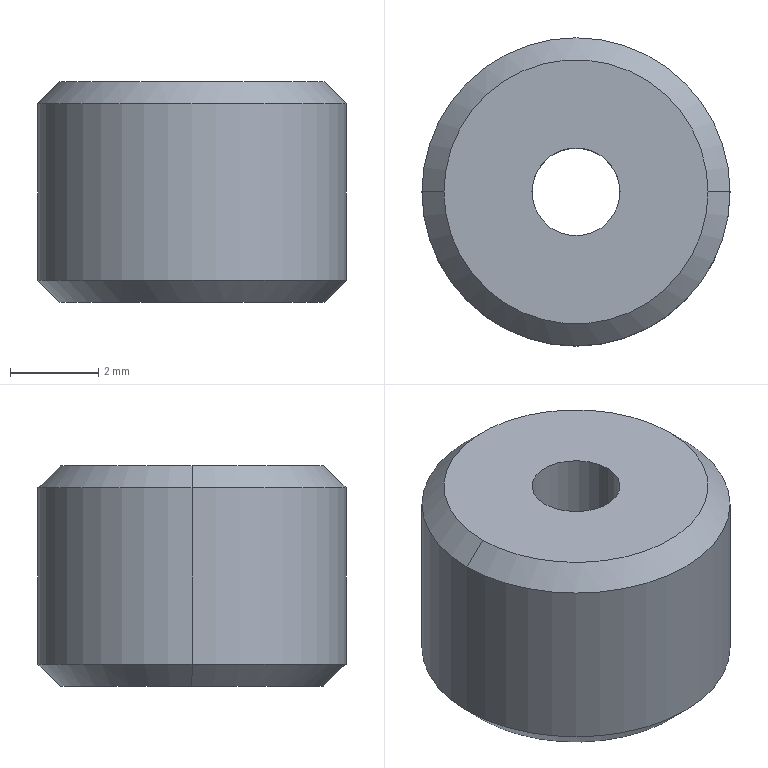Part | SolidWorks | features Chamfer 1, Extrusion 1, ICE 1 | 1 solid | 10 faces | box 7 x 7 x 5 mm | volume 171.479 mm3 | cone 4 | cylinder 4 | plane 2 | commonest cylinder face diameters 2 x2 7 x2
STEP:
#1=CARTESIAN_POINT('',(3.,0.,5.));
#2=VERTEX_POINT('',#1);
#3=CARTESIAN_POINT('',(-3.,0.,5.));
#4=VERTEX_POINT('',#3);
#5=CARTESIAN_POINT('',(0.,0.,5.));
#6=DIRECTION('',(0.,0.,1.));
#7=DIRECTION('',(1.,0.,0.));
#8=AXIS2_PLACEMENT_3D('',#5,#6,#7);
#9=CIRCLE('',#8,3.);
#10=EDGE_CURVE('',#2,#4,#9,.T.);
#11=ORIENTED_EDGE('',*,*,#10,.F.);
#12=CARTESIAN_POINT('',(3.5,0.,4.5));
#13=VERTEX_POINT('',#12);
#14=CARTESIAN_POINT('',(3.,0.,5.));
#15=DIRECTION('',(0.7071,0.,-0.7071));
#16=VECTOR('',#15,1000.);
#17=LINE('',#14,#16);
#18=EDGE_CURVE('',#2,#13,#17,.T.);
#19=ORIENTED_EDGE('',*,*,#18,.T.);
#20=CARTESIAN_POINT('',(-3.5,0.,4.5));
#21=VERTEX_POINT('',#20);
#22=CARTESIAN_POINT('',(0.,0.,4.5));
#23=DIRECTION('',(0.,0.,-1.));
#24=DIRECTION('',(1.,0.,0.));
#25=AXIS2_PLACEMENT_3D('',#22,#23,#24);
#26=CIRCLE('',#25,3.5);
#27=EDGE_CURVE('',#21,#13,#26,.T.);
#28=ORIENTED_EDGE('',*,*,#27,.F.);
#29=CARTESIAN_POINT('',(-3.,0.,5.));
#30=DIRECTION('',(-0.7071,0.,-0.7071));
#31=VECTOR('',#30,1000.);
#32=LINE('',#29,#31);
#33=EDGE_CURVE('',#4,#21,#32,.T.);
#34=ORIENTED_EDGE('',*,*,#33,.F.);
#35=EDGE_LOOP('',(#11,#19,#28,#34));
#36=FACE_OUTER_BOUND('',#35,.T.);
#37=CARTESIAN_POINT('',(0.,0.,5.));
#38=DIRECTION('',(0.,0.,-1.));
#39=DIRECTION('',(-1.,0.,0.));
#40=AXIS2_PLACEMENT_3D('',#37,#38,#39);
#41=CONICAL_SURFACE('',#40,3.,0.7854);
#42=ADVANCED_FACE('',(#36),#41,.T.);
#43=CARTESIAN_POINT('',(-3.,0.,0.));
#44=VERTEX_POINT('',#43);
#45=CARTESIAN_POINT('',(3.,0.,0.));
#46=VERTEX_POINT('',#45);
#47=CARTESIAN_POINT('',(0.,0.,0.));
#48=DIRECTION('',(0.,0.,-1.));
#49=DIRECTION('',(1.,0.,0.));
#50=AXIS2_PLACEMENT_3D('',#47,#48,#49);
#51=CIRCLE('',#50,3.);
#52=EDGE_CURVE('',#44,#46,#51,.T.);
#53=ORIENTED_EDGE('',*,*,#52,.F.);
#54=CARTESIAN_POINT('',(-3.5,0.,0.5));
#55=VERTEX_POINT('',#54);
#56=CARTESIAN_POINT('',(-3.5,0.,0.5));
#57=DIRECTION('',(-0.7071,0.,0.7071));
#58=VECTOR('',#57,1000.);
#59=LINE('',#56,#58);
#60=EDGE_CURVE('',#44,#55,#59,.T.);
#61=ORIENTED_EDGE('',*,*,#60,.T.);
#62=CARTESIAN_POINT('',(3.5,0.,0.5));
#63=VERTEX_POINT('',#62);
#64=CARTESIAN_POINT('',(0.,0.,0.5));
#65=DIRECTION('',(0.,0.,1.));
#66=DIRECTION('',(1.,0.,0.));
#67=AXIS2_PLACEMENT_3D('',#64,#65,#66);
#68=CIRCLE('',#67,3.5);
#69=EDGE_CURVE('',#63,#55,#68,.T.);
#70=ORIENTED_EDGE('',*,*,#69,.F.);
#71=CARTESIAN_POINT('',(3.5,0.,0.5));
#72=DIRECTION('',(0.7071,0.,0.7071));
#73=VECTOR('',#72,1000.);
#74=LINE('',#71,#73);
#75=EDGE_CURVE('',#46,#63,#74,.T.);
#76=ORIENTED_EDGE('',*,*,#75,.F.);
#77=EDGE_LOOP('',(#53,#61,#70,#76));
#78=FACE_OUTER_BOUND('',#77,.T.);
#79=CARTESIAN_POINT('',(0.,0.,0.5));
#80=DIRECTION('',(0.,0.,1.));
#81=DIRECTION('',(1.,0.,0.));
#82=AXIS2_PLACEMENT_3D('',#79,#80,#81);
#83=CONICAL_SURFACE('',#82,3.5,0.7854);
#84=ADVANCED_FACE('',(#78),#83,.T.);
#85=CARTESIAN_POINT('',(-1.,0.,0.));
#86=VERTEX_POINT('',#85);
#87=CARTESIAN_POINT('',(1.,0.,0.));
#88=VERTEX_POINT('',#87);
#89=CARTESIAN_POINT('',(0.,0.,0.));
#90=DIRECTION('',(0.,0.,1.));
#91=DIRECTION('',(1.,0.,0.));
#92=AXIS2_PLACEMENT_3D('',#89,#90,#91);
#93=CIRCLE('',#92,1.);
#94=EDGE_CURVE('',#86,#88,#93,.T.);
#95=ORIENTED_EDGE('',*,*,#94,.F.);
#96=CARTESIAN_POINT('',(-1.,0.,5.));
#97=VERTEX_POINT('',#96);
#98=CARTESIAN_POINT('',(-1.,0.,-6.));
#99=DIRECTION('',(0.,0.,1.));
#100=VECTOR('',#99,1000.);
#101=LINE('',#98,#100);
#102=EDGE_CURVE('',#86,#97,#101,.T.);
#103=ORIENTED_EDGE('',*,*,#102,.T.);
#104=CARTESIAN_POINT('',(1.,0.,5.));
#105=VERTEX_POINT('',#104);
#106=CARTESIAN_POINT('',(0.,0.,5.));
#107=DIRECTION('',(0.,0.,1.));
#108=DIRECTION('',(1.,0.,0.));
#109=AXIS2_PLACEMENT_3D('',#106,#107,#108);
#110=CIRCLE('',#109,1.);
#111=EDGE_CURVE('',#97,#105,#110,.T.);
#112=ORIENTED_EDGE('',*,*,#111,.T.);
#113=CARTESIAN_POINT('',(1.,0.,-6.));
#114=DIRECTION('',(0.,0.,1.));
#115=VECTOR('',#114,1000.);
#116=LINE('',#113,#115);
#117=EDGE_CURVE('',#88,#105,#116,.T.);
#118=ORIENTED_EDGE('',*,*,#117,.F.);
#119=EDGE_LOOP('',(#95,#103,#112,#118));
#120=FACE_OUTER_BOUND('',#119,.T.);
#121=CARTESIAN_POINT('',(0.,0.,-6.));
#122=DIRECTION('',(0.,0.,1.));
#123=DIRECTION('',(1.,0.,0.));
#124=AXIS2_PLACEMENT_3D('',#121,#122,#123);
#125=CYLINDRICAL_SURFACE('',#124,1.);
#126=ADVANCED_FACE('',(#120),#125,.F.);
#127=ORIENTED_EDGE('',*,*,#27,.T.);
#128=CARTESIAN_POINT('',(3.5,0.,5.));
#129=DIRECTION('',(0.,0.,-1.));
#130=VECTOR('',#129,1000.);
#131=LINE('',#128,#130);
#132=EDGE_CURVE('',#13,#63,#131,.T.);
#133=ORIENTED_EDGE('',*,*,#132,.T.);
#134=ORIENTED_EDGE('',*,*,#69,.T.);
#135=CARTESIAN_POINT('',(-3.5,0.,5.));
#136=DIRECTION('',(0.,0.,-1.));
#137=VECTOR('',#136,1000.);
#138=LINE('',#135,#137);
#139=EDGE_CURVE('',#21,#55,#138,.T.);
#140=ORIENTED_EDGE('',*,*,#139,.F.);
#141=EDGE_LOOP('',(#127,#133,#134,#140));
#142=FACE_OUTER_BOUND('',#141,.T.);
#143=CARTESIAN_POINT('',(0.,0.,5.));
#144=DIRECTION('',(0.,0.,-1.));
#145=DIRECTION('',(-1.,0.,0.));
#146=AXIS2_PLACEMENT_3D('',#143,#144,#145);
#147=CYLINDRICAL_SURFACE('',#146,3.5);
#148=ADVANCED_FACE('',(#142),#147,.T.);
#149=ORIENTED_EDGE('',*,*,#132,.F.);
#150=CARTESIAN_POINT('',(0.,0.,4.5));
#151=DIRECTION('',(0.,0.,-1.));
#152=DIRECTION('',(1.,0.,0.));
#153=AXIS2_PLACEMENT_3D('',#150,#151,#152);
#154=CIRCLE('',#153,3.5);
#155=EDGE_CURVE('',#13,#21,#154,.T.);
#156=ORIENTED_EDGE('',*,*,#155,.T.);
#157=ORIENTED_EDGE('',*,*,#139,.T.);
#158=CARTESIAN_POINT('',(0.,0.,0.5));
#159=DIRECTION('',(0.,0.,1.));
#160=DIRECTION('',(1.,0.,0.));
#161=AXIS2_PLACEMENT_3D('',#158,#159,#160);
#162=CIRCLE('',#161,3.5);
#163=EDGE_CURVE('',#55,#63,#162,.T.);
#164=ORIENTED_EDGE('',*,*,#163,.T.);
#165=EDGE_LOOP('',(#149,#156,#157,#164));
#166=FACE_OUTER_BOUND('',#165,.T.);
#167=CARTESIAN_POINT('',(0.,0.,5.));
#168=DIRECTION('',(0.,0.,-1.));
#169=DIRECTION('',(-1.,0.,0.));
#170=AXIS2_PLACEMENT_3D('',#167,#168,#169);
#171=CYLINDRICAL_SURFACE('',#170,3.5);
#172=ADVANCED_FACE('',(#166),#171,.T.);
#173=CARTESIAN_POINT('',(0.,0.,5.));
#174=DIRECTION('',(0.,0.,1.));
#175=DIRECTION('',(1.,0.,0.));
#176=AXIS2_PLACEMENT_3D('',#173,#174,#175);
#177=CIRCLE('',#176,3.);
#178=EDGE_CURVE('',#4,#2,#177,.T.);
#179=ORIENTED_EDGE('',*,*,#178,.T.);
#180=ORIENTED_EDGE('',*,*,#10,.T.);
#181=EDGE_LOOP('',(#179,#180));
#182=FACE_OUTER_BOUND('',#181,.T.);
#183=CARTESIAN_POINT('',(0.,0.,5.));
#184=DIRECTION('',(0.,0.,1.));
#185=DIRECTION('',(1.,0.,0.));
#186=AXIS2_PLACEMENT_3D('',#183,#184,#185);
#187=CIRCLE('',#186,1.);
#188=EDGE_CURVE('',#105,#97,#187,.T.);
#189=ORIENTED_EDGE('',*,*,#188,.F.);
#190=ORIENTED_EDGE('',*,*,#111,.F.);
#191=EDGE_LOOP('',(#189,#190));
#192=FACE_BOUND('',#191,.T.);
#193=CARTESIAN_POINT('',(0.,0.,5.));
#194=DIRECTION('',(0.,0.,1.));
#195=DIRECTION('',(1.,0.,0.));
#196=AXIS2_PLACEMENT_3D('',#193,#194,#195);
#197=PLANE('',#196);
#198=ADVANCED_FACE('',(#182,#192),#197,.T.);
#199=CARTESIAN_POINT('',(0.,0.,0.));
#200=DIRECTION('',(0.,0.,-1.));
#201=DIRECTION('',(1.,0.,0.));
#202=AXIS2_PLACEMENT_3D('',#199,#200,#201);
#203=CIRCLE('',#202,3.);
#204=EDGE_CURVE('',#46,#44,#203,.T.);
#205=ORIENTED_EDGE('',*,*,#204,.T.);
#206=ORIENTED_EDGE('',*,*,#52,.T.);
#207=EDGE_LOOP('',(#205,#206));
#208=FACE_OUTER_BOUND('',#207,.T.);
#209=CARTESIAN_POINT('',(0.,0.,0.));
#210=DIRECTION('',(0.,0.,1.));
#211=DIRECTION('',(1.,0.,0.));
#212=AXIS2_PLACEMENT_3D('',#209,#210,#211);
#213=CIRCLE('',#212,1.);
#214=EDGE_CURVE('',#88,#86,#213,.T.);
#215=ORIENTED_EDGE('',*,*,#214,.T.);
#216=ORIENTED_EDGE('',*,*,#94,.T.);
#217=EDGE_LOOP('',(#215,#216));
#218=FACE_BOUND('',#217,.T.);
#219=CARTESIAN_POINT('',(0.,0.,0.));
#220=DIRECTION('',(0.,0.,1.));
#221=DIRECTION('',(1.,0.,0.));
#222=AXIS2_PLACEMENT_3D('',#219,#220,#221);
#223=PLANE('',#222);
#224=ADVANCED_FACE('',(#208,#218),#223,.F.);
#225=ORIENTED_EDGE('',*,*,#102,.F.);
#226=ORIENTED_EDGE('',*,*,#214,.F.);
#227=ORIENTED_EDGE('',*,*,#117,.T.);
#228=ORIENTED_EDGE('',*,*,#188,.T.);
#229=EDGE_LOOP('',(#225,#226,#227,#228));
#230=FACE_OUTER_BOUND('',#229,.T.);
#231=CARTESIAN_POINT('',(0.,0.,-6.));
#232=DIRECTION('',(0.,0.,1.));
#233=DIRECTION('',(1.,0.,0.));
#234=AXIS2_PLACEMENT_3D('',#231,#232,#233);
#235=CYLINDRICAL_SURFACE('',#234,1.);
#236=ADVANCED_FACE('',(#230),#235,.F.);
#237=ORIENTED_EDGE('',*,*,#60,.F.);
#238=ORIENTED_EDGE('',*,*,#204,.F.);
#239=ORIENTED_EDGE('',*,*,#75,.T.);
#240=ORIENTED_EDGE('',*,*,#163,.F.);
#241=EDGE_LOOP('',(#237,#238,#239,#240));
#242=FACE_OUTER_BOUND('',#241,.T.);
#243=CARTESIAN_POINT('',(0.,0.,0.5));
#244=DIRECTION('',(0.,0.,1.));
#245=DIRECTION('',(1.,0.,0.));
#246=AXIS2_PLACEMENT_3D('',#243,#244,#245);
#247=CONICAL_SURFACE('',#246,3.5,0.7854);
#248=ADVANCED_FACE('',(#242),#247,.T.);
#249=ORIENTED_EDGE('',*,*,#18,.F.);
#250=ORIENTED_EDGE('',*,*,#178,.F.);
#251=ORIENTED_EDGE('',*,*,#33,.T.);
#252=ORIENTED_EDGE('',*,*,#155,.F.);
#253=EDGE_LOOP('',(#249,#250,#251,#252));
#254=FACE_OUTER_BOUND('',#253,.T.);
#255=CARTESIAN_POINT('',(0.,0.,5.));
#256=DIRECTION('',(0.,0.,-1.));
#257=DIRECTION('',(-1.,0.,0.));
#258=AXIS2_PLACEMENT_3D('',#255,#256,#257);
#259=CONICAL_SURFACE('',#258,3.,0.7854);
#260=ADVANCED_FACE('',(#254),#259,.T.);
#261=CLOSED_SHELL('',(#42,#84,#126,#148,#172,#198,#224,#236,#248,#260));
#262=MANIFOLD_SOLID_BREP('',#261);
#263=CARTESIAN_POINT('',(0.,0.,0.));
#264=DIRECTION('',(0.,0.,1.));
#265=DIRECTION('',(1.,0.,0.));
#266=AXIS2_PLACEMENT_3D('',#263,#264,#265);
#267=(LENGTH_UNIT()NAMED_UNIT(*)SI_UNIT(.MILLI.,.METRE.));
#268=UNCERTAINTY_MEASURE_WITH_UNIT(LENGTH_MEASURE(0.00001),#267,'','');
#269=(NAMED_UNIT(*)PLANE_ANGLE_UNIT()SI_UNIT($,.RADIAN.));
#270=(NAMED_UNIT(*)SI_UNIT($,.STERADIAN.)SOLID_ANGLE_UNIT());
#271=(GEOMETRIC_REPRESENTATION_CONTEXT(3)GLOBAL_UNCERTAINTY_ASSIGNED_CONTEXT((#268))GLOBAL_UNIT_ASSIGNED_CONTEXT((#267,#269,#270))REPRESENTATION_CONTEXT('',''));
#272=ADVANCED_BREP_SHAPE_REPRESENTATION('',(#262,#266),#271);